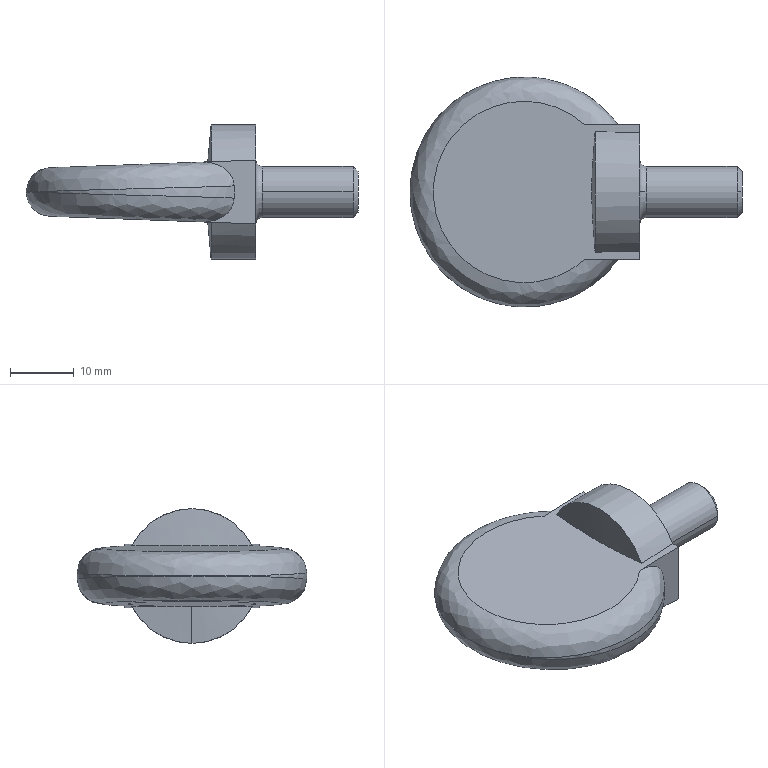Part | NX | features BREP 1 | 1 solid | 23 faces | box 52 x 36 x 21.1 mm | volume 10161 mm3 | cylinder 7 | plane 7 | cone 5 | torus 2 | spline 2 | commonest cylinder face diameters 8 x2 21.1 x2 36 x2 20 x1